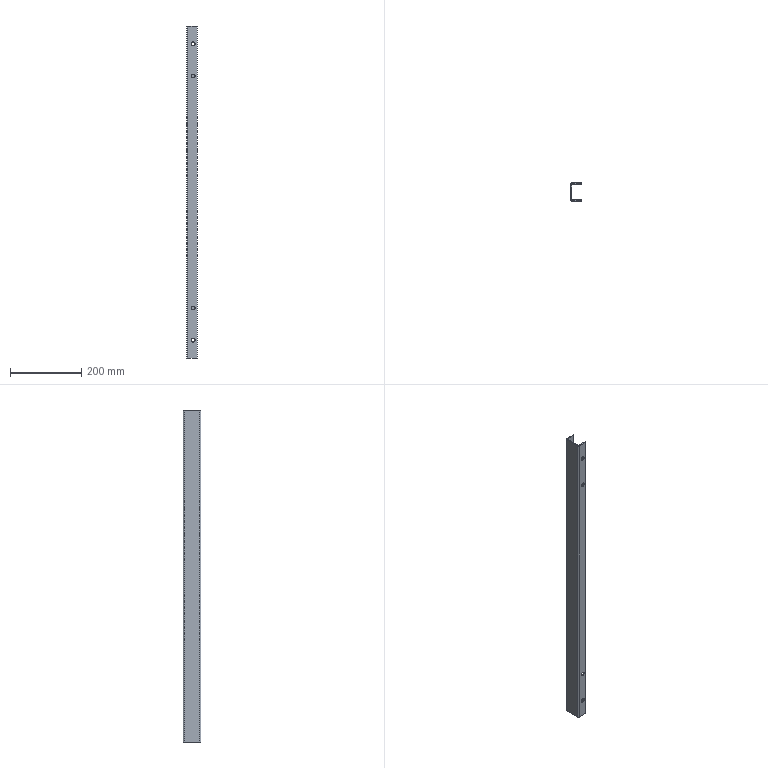Part | 1 solid | 55 faces | box 30 x 50 x 929 mm | volume 280462 mm3 | plane 28 | cylinder 27 | commonest cylinder face diameters 10 x15 11 x8 0.4 x2 6.4 x2